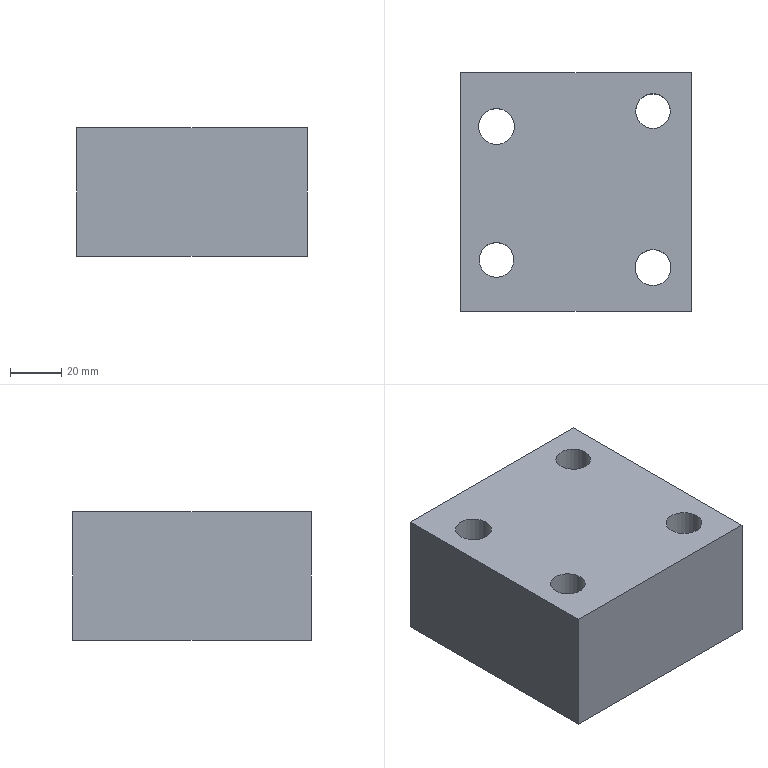Part | STEP file | lll_id3162_x_t | 1 solid | 12 faces | box 90 x 93 x 50 mm | volume 387590 mm3 | plane 6 | cylinder 5 | cone 1 | commonest cylinder face diameters 13.509 x2 14 x2 8.5 x1
STEP:
#1=CARTESIAN_POINT('',(473.754,320.75,142.5));
#2=VERTEX_POINT('',#1);
#3=CARTESIAN_POINT('',(467.,320.75,142.5));
#4=DIRECTION('',(0.,0.,-1.));
#5=DIRECTION('',(1.,0.,0.));
#6=AXIS2_PLACEMENT_3D('',#3,#4,#5);
#7=CIRCLE('',#6,6.755);
#8=EDGE_CURVE('',#2,#2,#7,.T.);
#9=ORIENTED_EDGE('',*,*,#8,.T.);
#10=EDGE_LOOP('',(#9));
#11=FACE_BOUND('',#10,.T.);
#12=CARTESIAN_POINT('',(412.754,262.75,142.5));
#13=VERTEX_POINT('',#12);
#14=CARTESIAN_POINT('',(406.,262.75,142.5));
#15=DIRECTION('',(0.,0.,-1.));
#16=DIRECTION('',(1.,0.,0.));
#17=AXIS2_PLACEMENT_3D('',#14,#15,#16);
#18=CIRCLE('',#17,6.755);
#19=EDGE_CURVE('',#13,#13,#18,.T.);
#20=ORIENTED_EDGE('',*,*,#19,.T.);
#21=EDGE_LOOP('',(#20));
#22=FACE_BOUND('',#21,.T.);
#23=CARTESIAN_POINT('',(392.,335.75,142.5));
#24=VERTEX_POINT('',#23);
#25=CARTESIAN_POINT('',(482.,335.75,142.5));
#26=VERTEX_POINT('',#25);
#27=CARTESIAN_POINT('',(437.,335.75,142.5));
#28=DIRECTION('',(1.,0.,0.));
#29=VECTOR('',#28,1.);
#30=LINE('',#27,#29);
#31=EDGE_CURVE('',#24,#26,#30,.T.);
#32=ORIENTED_EDGE('',*,*,#31,.F.);
#33=CARTESIAN_POINT('',(392.,242.75,142.5));
#34=VERTEX_POINT('',#33);
#35=CARTESIAN_POINT('',(392.,291.75,142.5));
#36=DIRECTION('',(0.,1.,0.));
#37=VECTOR('',#36,1.);
#38=LINE('',#35,#37);
#39=EDGE_CURVE('',#34,#24,#38,.T.);
#40=ORIENTED_EDGE('',*,*,#39,.F.);
#41=CARTESIAN_POINT('',(482.,242.75,142.5));
#42=VERTEX_POINT('',#41);
#43=CARTESIAN_POINT('',(437.,242.75,142.5));
#44=DIRECTION('',(-1.,0.,0.));
#45=VECTOR('',#44,1.);
#46=LINE('',#43,#45);
#47=EDGE_CURVE('',#42,#34,#46,.T.);
#48=ORIENTED_EDGE('',*,*,#47,.F.);
#49=CARTESIAN_POINT('',(482.,291.75,142.5));
#50=DIRECTION('',(0.,-1.,0.));
#51=VECTOR('',#50,1.);
#52=LINE('',#49,#51);
#53=EDGE_CURVE('',#26,#42,#52,.T.);
#54=ORIENTED_EDGE('',*,*,#53,.F.);
#55=EDGE_LOOP('',(#32,#40,#48,#54));
#56=FACE_BOUND('',#55,.T.);
#57=CARTESIAN_POINT('',(413.,314.75,142.5));
#58=VERTEX_POINT('',#57);
#59=CARTESIAN_POINT('',(406.,314.75,142.5));
#60=DIRECTION('',(0.,0.,-1.));
#61=DIRECTION('',(1.,0.,0.));
#62=AXIS2_PLACEMENT_3D('',#59,#60,#61);
#63=CIRCLE('',#62,7.);
#64=EDGE_CURVE('',#58,#58,#63,.T.);
#65=ORIENTED_EDGE('',*,*,#64,.T.);
#66=EDGE_LOOP('',(#65));
#67=FACE_BOUND('',#66,.T.);
#68=CARTESIAN_POINT('',(474.,259.75,142.5));
#69=VERTEX_POINT('',#68);
#70=CARTESIAN_POINT('',(467.,259.75,142.5));
#71=DIRECTION('',(0.,0.,-1.));
#72=DIRECTION('',(1.,0.,0.));
#73=AXIS2_PLACEMENT_3D('',#70,#71,#72);
#74=CIRCLE('',#73,7.);
#75=EDGE_CURVE('',#69,#69,#74,.T.);
#76=ORIENTED_EDGE('',*,*,#75,.T.);
#77=EDGE_LOOP('',(#76));
#78=FACE_BOUND('',#77,.T.);
#79=CARTESIAN_POINT('',(42.419,-273.704,142.5));
#80=DIRECTION('',(0.,0.,1.));
#81=DIRECTION('',(-1.,0.,0.));
#82=AXIS2_PLACEMENT_3D('',#79,#80,#81);
#83=PLANE('',#82);
#84=ADVANCED_FACE('',(#11,#22,#56,#67,#78),#83,.T.);
#85=CARTESIAN_POINT('',(441.25,273.5,92.5));
#86=VERTEX_POINT('',#85);
#87=CARTESIAN_POINT('',(437.,273.5,92.5));
#88=DIRECTION('',(0.,0.,1.));
#89=DIRECTION('',(1.,0.,0.));
#90=AXIS2_PLACEMENT_3D('',#87,#88,#89);
#91=CIRCLE('',#90,4.25);
#92=EDGE_CURVE('',#86,#86,#91,.T.);
#93=ORIENTED_EDGE('',*,*,#92,.T.);
#94=EDGE_LOOP('',(#93));
#95=FACE_BOUND('',#94,.T.);
#96=CARTESIAN_POINT('',(399.,314.75,92.5));
#97=VERTEX_POINT('',#96);
#98=CARTESIAN_POINT('',(406.,314.75,92.5));
#99=DIRECTION('',(0.,0.,1.));
#100=DIRECTION('',(-1.,0.,0.));
#101=AXIS2_PLACEMENT_3D('',#98,#99,#100);
#102=CIRCLE('',#101,7.);
#103=EDGE_CURVE('',#97,#97,#102,.T.);
#104=ORIENTED_EDGE('',*,*,#103,.T.);
#105=EDGE_LOOP('',(#104));
#106=FACE_BOUND('',#105,.T.);
#107=CARTESIAN_POINT('',(412.754,262.75,92.5));
#108=VERTEX_POINT('',#107);
#109=CARTESIAN_POINT('',(406.,262.75,92.5));
#110=DIRECTION('',(0.,0.,-1.));
#111=DIRECTION('',(1.,0.,0.));
#112=AXIS2_PLACEMENT_3D('',#109,#110,#111);
#113=CIRCLE('',#112,6.755);
#114=EDGE_CURVE('',#108,#108,#113,.T.);
#115=ORIENTED_EDGE('',*,*,#114,.F.);
#116=EDGE_LOOP('',(#115));
#117=FACE_BOUND('',#116,.T.);
#118=CARTESIAN_POINT('',(392.,335.75,92.5));
#119=VERTEX_POINT('',#118);
#120=CARTESIAN_POINT('',(392.,242.75,92.5));
#121=VERTEX_POINT('',#120);
#122=CARTESIAN_POINT('',(392.,291.75,92.5));
#123=DIRECTION('',(0.,-1.,0.));
#124=VECTOR('',#123,1.);
#125=LINE('',#122,#124);
#126=EDGE_CURVE('',#119,#121,#125,.T.);
#127=ORIENTED_EDGE('',*,*,#126,.F.);
#128=CARTESIAN_POINT('',(482.,335.75,92.5));
#129=VERTEX_POINT('',#128);
#130=CARTESIAN_POINT('',(437.,335.75,92.5));
#131=DIRECTION('',(-1.,0.,0.));
#132=VECTOR('',#131,1.);
#133=LINE('',#130,#132);
#134=EDGE_CURVE('',#129,#119,#133,.T.);
#135=ORIENTED_EDGE('',*,*,#134,.F.);
#136=CARTESIAN_POINT('',(482.,242.75,92.5));
#137=VERTEX_POINT('',#136);
#138=CARTESIAN_POINT('',(482.,291.75,92.5));
#139=DIRECTION('',(0.,1.,0.));
#140=VECTOR('',#139,1.);
#141=LINE('',#138,#140);
#142=EDGE_CURVE('',#137,#129,#141,.T.);
#143=ORIENTED_EDGE('',*,*,#142,.F.);
#144=CARTESIAN_POINT('',(437.,242.75,92.5));
#145=DIRECTION('',(1.,0.,0.));
#146=VECTOR('',#145,1.);
#147=LINE('',#144,#146);
#148=EDGE_CURVE('',#121,#137,#147,.T.);
#149=ORIENTED_EDGE('',*,*,#148,.F.);
#150=EDGE_LOOP('',(#127,#135,#143,#149));
#151=FACE_BOUND('',#150,.T.);
#152=CARTESIAN_POINT('',(473.754,320.75,92.5));
#153=VERTEX_POINT('',#152);
#154=CARTESIAN_POINT('',(467.,320.75,92.5));
#155=DIRECTION('',(0.,0.,-1.));
#156=DIRECTION('',(1.,0.,0.));
#157=AXIS2_PLACEMENT_3D('',#154,#155,#156);
#158=CIRCLE('',#157,6.755);
#159=EDGE_CURVE('',#153,#153,#158,.T.);
#160=ORIENTED_EDGE('',*,*,#159,.F.);
#161=EDGE_LOOP('',(#160));
#162=FACE_BOUND('',#161,.T.);
#163=CARTESIAN_POINT('',(474.,259.75,92.5));
#164=VERTEX_POINT('',#163);
#165=CARTESIAN_POINT('',(467.,259.75,92.5));
#166=DIRECTION('',(0.,0.,1.));
#167=DIRECTION('',(1.,0.,0.));
#168=AXIS2_PLACEMENT_3D('',#165,#166,#167);
#169=CIRCLE('',#168,7.);
#170=EDGE_CURVE('',#164,#164,#169,.T.);
#171=ORIENTED_EDGE('',*,*,#170,.T.);
#172=EDGE_LOOP('',(#171));
#173=FACE_BOUND('',#172,.T.);
#174=CARTESIAN_POINT('',(437.,291.75,92.5));
#175=DIRECTION('',(0.,0.,-1.));
#176=DIRECTION('',(1.,0.,0.));
#177=AXIS2_PLACEMENT_3D('',#174,#175,#176);
#178=PLANE('',#177);
#179=ADVANCED_FACE('',(#95,#106,#117,#151,#162,#173),#178,.T.);
#180=CARTESIAN_POINT('',(392.,335.75,92.5));
#181=DIRECTION('',(0.,0.,1.));
#182=VECTOR('',#181,1.);
#183=LINE('',#180,#182);
#184=EDGE_CURVE('',#119,#24,#183,.T.);
#185=ORIENTED_EDGE('',*,*,#184,.T.);
#186=ORIENTED_EDGE('',*,*,#31,.T.);
#187=CARTESIAN_POINT('',(482.,335.75,92.5));
#188=DIRECTION('',(0.,0.,1.));
#189=VECTOR('',#188,1.);
#190=LINE('',#187,#189);
#191=EDGE_CURVE('',#129,#26,#190,.T.);
#192=ORIENTED_EDGE('',*,*,#191,.F.);
#193=ORIENTED_EDGE('',*,*,#134,.T.);
#194=EDGE_LOOP('',(#185,#186,#192,#193));
#195=FACE_OUTER_BOUND('',#194,.T.);
#196=CARTESIAN_POINT('',(437.,335.75,92.5));
#197=DIRECTION('',(0.,1.,0.));
#198=DIRECTION('',(0.,0.,-1.));
#199=AXIS2_PLACEMENT_3D('',#196,#197,#198);
#200=PLANE('',#199);
#201=ADVANCED_FACE('',(#195),#200,.T.);
#202=ORIENTED_EDGE('',*,*,#191,.T.);
#203=ORIENTED_EDGE('',*,*,#53,.T.);
#204=CARTESIAN_POINT('',(482.,242.75,60.5));
#205=DIRECTION('',(0.,0.,1.));
#206=VECTOR('',#205,1.);
#207=LINE('',#204,#206);
#208=EDGE_CURVE('',#137,#42,#207,.T.);
#209=ORIENTED_EDGE('',*,*,#208,.F.);
#210=ORIENTED_EDGE('',*,*,#142,.T.);
#211=EDGE_LOOP('',(#202,#203,#209,#210));
#212=FACE_OUTER_BOUND('',#211,.T.);
#213=CARTESIAN_POINT('',(482.,291.75,92.5));
#214=DIRECTION('',(1.,0.,0.));
#215=DIRECTION('',(0.,0.,1.));
#216=AXIS2_PLACEMENT_3D('',#213,#214,#215);
#217=PLANE('',#216);
#218=ADVANCED_FACE('',(#212),#217,.T.);
#219=ORIENTED_EDGE('',*,*,#208,.T.);
#220=ORIENTED_EDGE('',*,*,#47,.T.);
#221=CARTESIAN_POINT('',(392.,242.75,92.5));
#222=DIRECTION('',(0.,0.,1.));
#223=VECTOR('',#222,1.);
#224=LINE('',#221,#223);
#225=EDGE_CURVE('',#121,#34,#224,.T.);
#226=ORIENTED_EDGE('',*,*,#225,.F.);
#227=ORIENTED_EDGE('',*,*,#148,.T.);
#228=EDGE_LOOP('',(#219,#220,#226,#227));
#229=FACE_OUTER_BOUND('',#228,.T.);
#230=CARTESIAN_POINT('',(437.,242.75,60.5));
#231=DIRECTION('',(0.,-1.,0.));
#232=DIRECTION('',(0.,0.,1.));
#233=AXIS2_PLACEMENT_3D('',#230,#231,#232);
#234=PLANE('',#233);
#235=ADVANCED_FACE('',(#229),#234,.T.);
#236=ORIENTED_EDGE('',*,*,#126,.T.);
#237=ORIENTED_EDGE('',*,*,#225,.T.);
#238=ORIENTED_EDGE('',*,*,#39,.T.);
#239=ORIENTED_EDGE('',*,*,#184,.F.);
#240=EDGE_LOOP('',(#236,#237,#238,#239));
#241=FACE_OUTER_BOUND('',#240,.T.);
#242=CARTESIAN_POINT('',(392.,291.75,92.5));
#243=DIRECTION('',(-1.,0.,0.));
#244=DIRECTION('',(0.,0.,-1.));
#245=AXIS2_PLACEMENT_3D('',#242,#243,#244);
#246=PLANE('',#245);
#247=ADVANCED_FACE('',(#241),#246,.T.);
#248=ORIENTED_EDGE('',*,*,#114,.T.);
#249=EDGE_LOOP('',(#248));
#250=FACE_BOUND('',#249,.T.);
#251=ORIENTED_EDGE('',*,*,#19,.F.);
#252=EDGE_LOOP('',(#251));
#253=FACE_BOUND('',#252,.T.);
#254=CARTESIAN_POINT('',(406.,262.75,57.5));
#255=DIRECTION('',(0.,0.,1.));
#256=DIRECTION('',(-1.,0.,0.));
#257=AXIS2_PLACEMENT_3D('',#254,#255,#256);
#258=CYLINDRICAL_SURFACE('',#257,6.755);
#259=ADVANCED_FACE('',(#250,#253),#258,.F.);
#260=ORIENTED_EDGE('',*,*,#64,.F.);
#261=EDGE_LOOP('',(#260));
#262=FACE_BOUND('',#261,.T.);
#263=ORIENTED_EDGE('',*,*,#103,.F.);
#264=EDGE_LOOP('',(#263));
#265=FACE_BOUND('',#264,.T.);
#266=CARTESIAN_POINT('',(406.,314.75,92.5));
#267=DIRECTION('',(0.,0.,1.));
#268=DIRECTION('',(-1.,0.,0.));
#269=AXIS2_PLACEMENT_3D('',#266,#267,#268);
#270=CYLINDRICAL_SURFACE('',#269,7.);
#271=ADVANCED_FACE('',(#262,#265),#270,.F.);
#272=ORIENTED_EDGE('',*,*,#159,.T.);
#273=EDGE_LOOP('',(#272));
#274=FACE_BOUND('',#273,.T.);
#275=ORIENTED_EDGE('',*,*,#8,.F.);
#276=EDGE_LOOP('',(#275));
#277=FACE_BOUND('',#276,.T.);
#278=CARTESIAN_POINT('',(467.,320.75,57.5));
#279=DIRECTION('',(0.,0.,1.));
#280=DIRECTION('',(1.,0.,0.));
#281=AXIS2_PLACEMENT_3D('',#278,#279,#280);
#282=CYLINDRICAL_SURFACE('',#281,6.755);
#283=ADVANCED_FACE('',(#274,#277),#282,.F.);
#284=ORIENTED_EDGE('',*,*,#75,.F.);
#285=EDGE_LOOP('',(#284));
#286=FACE_BOUND('',#285,.T.);
#287=ORIENTED_EDGE('',*,*,#170,.F.);
#288=EDGE_LOOP('',(#287));
#289=FACE_BOUND('',#288,.T.);
#290=CARTESIAN_POINT('',(467.,259.75,92.5));
#291=DIRECTION('',(0.,0.,1.));
#292=DIRECTION('',(1.,0.,0.));
#293=AXIS2_PLACEMENT_3D('',#290,#291,#292);
#294=CYLINDRICAL_SURFACE('',#293,7.);
#295=ADVANCED_FACE('',(#286,#289),#294,.F.);
#296=CARTESIAN_POINT('',(441.25,273.5,112.5));
#297=VERTEX_POINT('',#296);
#298=CARTESIAN_POINT('',(437.,273.5,112.5));
#299=DIRECTION('',(0.,0.,-1.));
#300=DIRECTION('',(1.,0.,0.));
#301=AXIS2_PLACEMENT_3D('',#298,#299,#300);
#302=CIRCLE('',#301,4.25);
#303=EDGE_CURVE('',#297,#297,#302,.T.);
#304=ORIENTED_EDGE('',*,*,#303,.T.);
#305=EDGE_LOOP('',(#304));
#306=FACE_BOUND('',#305,.T.);
#307=CARTESIAN_POINT('',(437.,273.5,115.054));
#308=VERTEX_POINT('',#307);
#309=VERTEX_LOOP('',#308);
#310=FACE_BOUND('',#309,.T.);
#311=CARTESIAN_POINT('',(437.,273.5,112.5));
#312=DIRECTION('',(0.,0.,-1.));
#313=DIRECTION('',(1.,0.,0.));
#314=AXIS2_PLACEMENT_3D('',#311,#312,#313);
#315=CONICAL_SURFACE('',#314,4.25,59.);
#316=ADVANCED_FACE('',(#306,#310),#315,.F.);
#317=ORIENTED_EDGE('',*,*,#303,.F.);
#318=EDGE_LOOP('',(#317));
#319=FACE_BOUND('',#318,.T.);
#320=ORIENTED_EDGE('',*,*,#92,.F.);
#321=EDGE_LOOP('',(#320));
#322=FACE_BOUND('',#321,.T.);
#323=CARTESIAN_POINT('',(437.,273.5,92.5));
#324=DIRECTION('',(0.,0.,1.));
#325=DIRECTION('',(-1.,0.,0.));
#326=AXIS2_PLACEMENT_3D('',#323,#324,#325);
#327=CYLINDRICAL_SURFACE('',#326,4.25);
#328=ADVANCED_FACE('',(#319,#322),#327,.F.);
#329=CLOSED_SHELL('',(#84,#179,#201,#218,#235,#247,#259,#271,#283,#295,#316,#328));
#330=MANIFOLD_SOLID_BREP('',#329);
#331=(LENGTH_UNIT()NAMED_UNIT(*)SI_UNIT(.MILLI.,.METRE.));
#332=UNCERTAINTY_MEASURE_WITH_UNIT(LENGTH_MEASURE(0.00002),#331,'','');
#333=(NAMED_UNIT(*)PLANE_ANGLE_UNIT()SI_UNIT($,.RADIAN.));
#334=PLANE_ANGLE_MEASURE_WITH_UNIT(PLANE_ANGLE_MEASURE(0.01745),#333);
#335=DIMENSIONAL_EXPONENTS(0.,0.,0.,0.,0.,0.,0.);
#336=(CONVERSION_BASED_UNIT('DEGREE',#334)NAMED_UNIT(#335)PLANE_ANGLE_UNIT());
#337=(NAMED_UNIT(*)SI_UNIT($,.STERADIAN.)SOLID_ANGLE_UNIT());
#338=(GEOMETRIC_REPRESENTATION_CONTEXT(3)GLOBAL_UNCERTAINTY_ASSIGNED_CONTEXT((#332))GLOBAL_UNIT_ASSIGNED_CONTEXT((#331,#336,#337))REPRESENTATION_CONTEXT('',''));
#339=ADVANCED_BREP_SHAPE_REPRESENTATION('',(#330),#338);